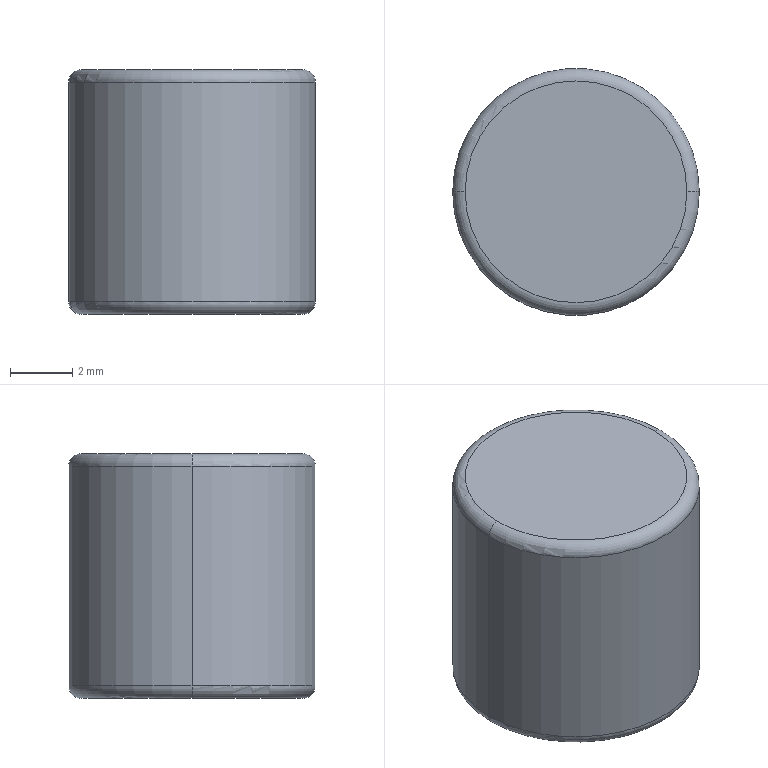Part | STEP file | RS40-AS-2LSR-T-266L-JR-Part-66 | 1 solid | 8 faces | box 7.92 x 7.92 x 7.85 mm | volume 385.066 mm3 | torus 4 | cylinder 2 | plane 2 | commonest cylinder face diameters 7.92 x2
STEP:
#1=CARTESIAN_POINT('',(1488.7,2.14,11.65));
#2=VERTEX_POINT('',#1);
#3=CARTESIAN_POINT('',(1480.78,2.14,11.65));
#4=VERTEX_POINT('',#3);
#5=CARTESIAN_POINT('',(1484.74,2.14,11.65));
#6=DIRECTION('',(0.,0.,-1.));
#7=DIRECTION('',(1.,0.,0.));
#8=AXIS2_PLACEMENT_3D('',#5,#6,#7);
#9=CIRCLE('',#8,3.96);
#10=EDGE_CURVE('',#2,#4,#9,.T.);
#11=ORIENTED_EDGE('',*,*,#10,.T.);
#12=CARTESIAN_POINT('',(1481.188,2.14,11.25));
#13=VERTEX_POINT('',#12);
#14=CARTESIAN_POINT('',(1481.184,2.14,11.654));
#15=DIRECTION('',(0.,-1.,0.));
#16=DIRECTION('',(1.,0.,0.));
#17=AXIS2_PLACEMENT_3D('',#14,#15,#16);
#18=CIRCLE('',#17,0.4038);
#19=EDGE_CURVE('',#4,#13,#18,.T.);
#20=ORIENTED_EDGE('',*,*,#19,.T.);
#21=CARTESIAN_POINT('',(1488.292,2.14,11.25));
#22=VERTEX_POINT('',#21);
#23=CARTESIAN_POINT('',(1484.74,2.14,11.25));
#24=DIRECTION('',(0.,0.,-1.));
#25=DIRECTION('',(1.,0.,0.));
#26=AXIS2_PLACEMENT_3D('',#23,#24,#25);
#27=CIRCLE('',#26,3.552);
#28=EDGE_CURVE('',#22,#13,#27,.T.);
#29=ORIENTED_EDGE('',*,*,#28,.F.);
#30=CARTESIAN_POINT('',(1488.296,2.14,11.654));
#31=DIRECTION('',(0.,1.,0.));
#32=DIRECTION('',(0.,0.,1.));
#33=AXIS2_PLACEMENT_3D('',#30,#31,#32);
#34=CIRCLE('',#33,0.4038);
#35=EDGE_CURVE('',#2,#22,#34,.T.);
#36=ORIENTED_EDGE('',*,*,#35,.F.);
#37=EDGE_LOOP('',(#11,#20,#29,#36));
#38=FACE_OUTER_BOUND('',#37,.T.);
#39=CARTESIAN_POINT('',(1484.74,2.14,11.654));
#40=DIRECTION('',(0.,0.,-1.));
#41=DIRECTION('',(1.,0.,0.));
#42=AXIS2_PLACEMENT_3D('',#39,#40,#41);
#43=TOROIDAL_SURFACE('',#42,3.556,0.4038);
#44=ADVANCED_FACE('',(#38),#43,.T.);
#45=CARTESIAN_POINT('',(1488.7,2.14,18.7));
#46=VERTEX_POINT('',#45);
#47=CARTESIAN_POINT('',(1480.78,2.14,18.7));
#48=VERTEX_POINT('',#47);
#49=CARTESIAN_POINT('',(1484.74,2.14,18.7));
#50=DIRECTION('',(0.,0.,-1.));
#51=DIRECTION('',(1.,0.,0.));
#52=AXIS2_PLACEMENT_3D('',#49,#50,#51);
#53=CIRCLE('',#52,3.96);
#54=EDGE_CURVE('',#46,#48,#53,.T.);
#55=ORIENTED_EDGE('',*,*,#54,.T.);
#56=CARTESIAN_POINT('',(1480.78,2.14,-2.725));
#57=DIRECTION('',(0.,0.,-1.));
#58=VECTOR('',#57,1000.);
#59=LINE('',#56,#58);
#60=EDGE_CURVE('',#48,#4,#59,.T.);
#61=ORIENTED_EDGE('',*,*,#60,.T.);
#62=ORIENTED_EDGE('',*,*,#10,.F.);
#63=CARTESIAN_POINT('',(1488.7,2.14,-2.725));
#64=DIRECTION('',(0.,0.,-1.));
#65=VECTOR('',#64,1000.);
#66=LINE('',#63,#65);
#67=EDGE_CURVE('',#46,#2,#66,.T.);
#68=ORIENTED_EDGE('',*,*,#67,.F.);
#69=EDGE_LOOP('',(#55,#61,#62,#68));
#70=FACE_OUTER_BOUND('',#69,.T.);
#71=CARTESIAN_POINT('',(1484.74,2.14,-2.725));
#72=DIRECTION('',(0.,0.,-1.));
#73=DIRECTION('',(1.,0.,0.));
#74=AXIS2_PLACEMENT_3D('',#71,#72,#73);
#75=CYLINDRICAL_SURFACE('',#74,3.96);
#76=ADVANCED_FACE('',(#70),#75,.T.);
#77=CARTESIAN_POINT('',(1488.3,2.14,19.1));
#78=VERTEX_POINT('',#77);
#79=CARTESIAN_POINT('',(1481.18,2.14,19.1));
#80=VERTEX_POINT('',#79);
#81=CARTESIAN_POINT('',(1484.74,2.14,19.1));
#82=DIRECTION('',(0.,0.,-1.));
#83=DIRECTION('',(1.,0.,0.));
#84=AXIS2_PLACEMENT_3D('',#81,#82,#83);
#85=CIRCLE('',#84,3.56);
#86=EDGE_CURVE('',#78,#80,#85,.T.);
#87=ORIENTED_EDGE('',*,*,#86,.T.);
#88=CARTESIAN_POINT('',(1481.18,2.14,18.7));
#89=DIRECTION('',(0.,-1.,0.));
#90=DIRECTION('',(1.,0.,0.));
#91=AXIS2_PLACEMENT_3D('',#88,#89,#90);
#92=CIRCLE('',#91,0.4);
#93=EDGE_CURVE('',#80,#48,#92,.T.);
#94=ORIENTED_EDGE('',*,*,#93,.T.);
#95=ORIENTED_EDGE('',*,*,#54,.F.);
#96=CARTESIAN_POINT('',(1488.3,2.14,18.7));
#97=DIRECTION('',(0.,1.,0.));
#98=DIRECTION('',(0.,0.,1.));
#99=AXIS2_PLACEMENT_3D('',#96,#97,#98);
#100=CIRCLE('',#99,0.4);
#101=EDGE_CURVE('',#78,#46,#100,.T.);
#102=ORIENTED_EDGE('',*,*,#101,.F.);
#103=EDGE_LOOP('',(#87,#94,#95,#102));
#104=FACE_OUTER_BOUND('',#103,.T.);
#105=CARTESIAN_POINT('',(1484.74,2.14,18.7));
#106=DIRECTION('',(0.,0.,-1.));
#107=DIRECTION('',(1.,0.,0.));
#108=AXIS2_PLACEMENT_3D('',#105,#106,#107);
#109=TOROIDAL_SURFACE('',#108,3.56,0.4);
#110=ADVANCED_FACE('',(#104),#109,.T.);
#111=ORIENTED_EDGE('',*,*,#86,.F.);
#112=CARTESIAN_POINT('',(1484.74,2.14,19.1));
#113=DIRECTION('',(0.,0.,-1.));
#114=DIRECTION('',(1.,0.,0.));
#115=AXIS2_PLACEMENT_3D('',#112,#113,#114);
#116=CIRCLE('',#115,3.56);
#117=EDGE_CURVE('',#80,#78,#116,.T.);
#118=ORIENTED_EDGE('',*,*,#117,.F.);
#119=EDGE_LOOP('',(#111,#118));
#120=FACE_OUTER_BOUND('',#119,.T.);
#121=CARTESIAN_POINT('',(1484.74,2.14,19.1));
#122=DIRECTION('',(0.,0.,-1.));
#123=DIRECTION('',(1.,0.,0.));
#124=AXIS2_PLACEMENT_3D('',#121,#122,#123);
#125=PLANE('',#124);
#126=ADVANCED_FACE('',(#120),#125,.F.);
#127=ORIENTED_EDGE('',*,*,#93,.F.);
#128=ORIENTED_EDGE('',*,*,#117,.T.);
#129=ORIENTED_EDGE('',*,*,#101,.T.);
#130=CARTESIAN_POINT('',(1484.74,2.14,18.7));
#131=DIRECTION('',(0.,0.,-1.));
#132=DIRECTION('',(1.,0.,0.));
#133=AXIS2_PLACEMENT_3D('',#130,#131,#132);
#134=CIRCLE('',#133,3.96);
#135=EDGE_CURVE('',#48,#46,#134,.T.);
#136=ORIENTED_EDGE('',*,*,#135,.F.);
#137=EDGE_LOOP('',(#127,#128,#129,#136));
#138=FACE_OUTER_BOUND('',#137,.T.);
#139=CARTESIAN_POINT('',(1484.74,2.14,18.7));
#140=DIRECTION('',(0.,0.,-1.));
#141=DIRECTION('',(1.,0.,0.));
#142=AXIS2_PLACEMENT_3D('',#139,#140,#141);
#143=TOROIDAL_SURFACE('',#142,3.56,0.4);
#144=ADVANCED_FACE('',(#138),#143,.T.);
#145=ORIENTED_EDGE('',*,*,#60,.F.);
#146=ORIENTED_EDGE('',*,*,#135,.T.);
#147=ORIENTED_EDGE('',*,*,#67,.T.);
#148=CARTESIAN_POINT('',(1484.74,2.14,11.65));
#149=DIRECTION('',(0.,0.,-1.));
#150=DIRECTION('',(1.,0.,0.));
#151=AXIS2_PLACEMENT_3D('',#148,#149,#150);
#152=CIRCLE('',#151,3.96);
#153=EDGE_CURVE('',#4,#2,#152,.T.);
#154=ORIENTED_EDGE('',*,*,#153,.F.);
#155=EDGE_LOOP('',(#145,#146,#147,#154));
#156=FACE_OUTER_BOUND('',#155,.T.);
#157=CARTESIAN_POINT('',(1484.74,2.14,-2.725));
#158=DIRECTION('',(0.,0.,-1.));
#159=DIRECTION('',(1.,0.,0.));
#160=AXIS2_PLACEMENT_3D('',#157,#158,#159);
#161=CYLINDRICAL_SURFACE('',#160,3.96);
#162=ADVANCED_FACE('',(#156),#161,.T.);
#163=ORIENTED_EDGE('',*,*,#19,.F.);
#164=ORIENTED_EDGE('',*,*,#153,.T.);
#165=ORIENTED_EDGE('',*,*,#35,.T.);
#166=CARTESIAN_POINT('',(1484.74,2.14,11.25));
#167=DIRECTION('',(0.,0.,-1.));
#168=DIRECTION('',(1.,0.,0.));
#169=AXIS2_PLACEMENT_3D('',#166,#167,#168);
#170=CIRCLE('',#169,3.552);
#171=EDGE_CURVE('',#13,#22,#170,.T.);
#172=ORIENTED_EDGE('',*,*,#171,.F.);
#173=EDGE_LOOP('',(#163,#164,#165,#172));
#174=FACE_OUTER_BOUND('',#173,.T.);
#175=CARTESIAN_POINT('',(1484.74,2.14,11.654));
#176=DIRECTION('',(0.,0.,-1.));
#177=DIRECTION('',(1.,0.,0.));
#178=AXIS2_PLACEMENT_3D('',#175,#176,#177);
#179=TOROIDAL_SURFACE('',#178,3.556,0.4038);
#180=ADVANCED_FACE('',(#174),#179,.T.);
#181=ORIENTED_EDGE('',*,*,#28,.T.);
#182=ORIENTED_EDGE('',*,*,#171,.T.);
#183=EDGE_LOOP('',(#181,#182));
#184=FACE_OUTER_BOUND('',#183,.T.);
#185=CARTESIAN_POINT('',(1481.188,2.14,11.25));
#186=DIRECTION('',(0.,0.,1.));
#187=DIRECTION('',(-1.,0.,0.));
#188=AXIS2_PLACEMENT_3D('',#185,#186,#187);
#189=PLANE('',#188);
#190=ADVANCED_FACE('',(#184),#189,.F.);
#191=CLOSED_SHELL('',(#44,#76,#110,#126,#144,#162,#180,#190));
#192=MANIFOLD_SOLID_BREP('',#191);
#193=CARTESIAN_POINT('',(0.,0.,0.));
#194=DIRECTION('',(0.,0.,1.));
#195=DIRECTION('',(1.,0.,0.));
#196=AXIS2_PLACEMENT_3D('',#193,#194,#195);
#197=(LENGTH_UNIT()NAMED_UNIT(*)SI_UNIT(.MILLI.,.METRE.));
#198=UNCERTAINTY_MEASURE_WITH_UNIT(LENGTH_MEASURE(0.00001),#197,'','');
#199=(NAMED_UNIT(*)PLANE_ANGLE_UNIT()SI_UNIT($,.RADIAN.));
#200=(NAMED_UNIT(*)SI_UNIT($,.STERADIAN.)SOLID_ANGLE_UNIT());
#201=(GEOMETRIC_REPRESENTATION_CONTEXT(3)GLOBAL_UNCERTAINTY_ASSIGNED_CONTEXT((#198))GLOBAL_UNIT_ASSIGNED_CONTEXT((#197,#199,#200))REPRESENTATION_CONTEXT('',''));
#202=ADVANCED_BREP_SHAPE_REPRESENTATION('',(#192,#196),#201);